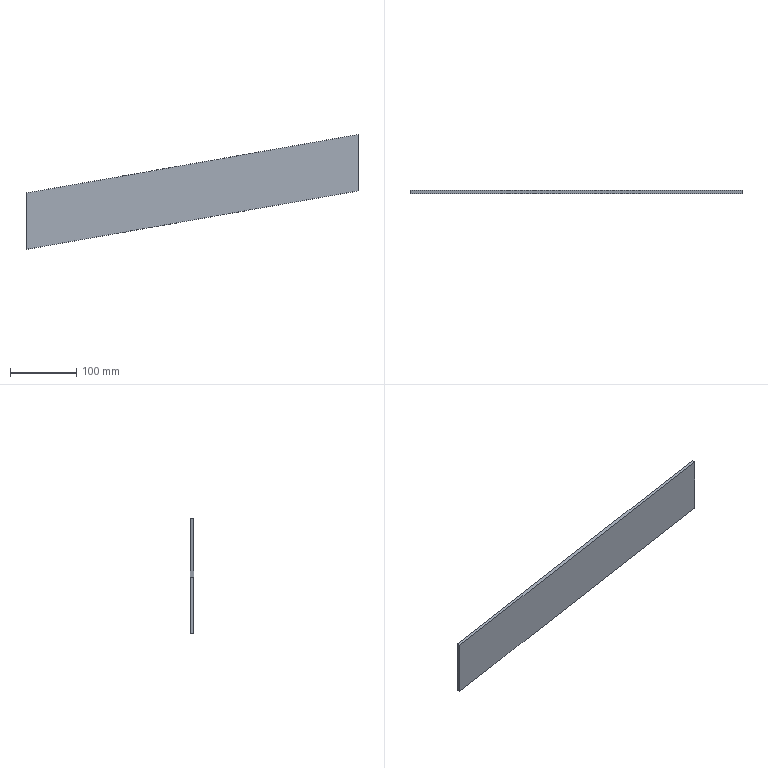Part | NX | features DATUM_CSYS 1, EXTRUDE 1, LINKED_CURVE 1 | 1 solid | 6 faces | box 500 x 5 x 173.163 mm | volume 212500 mm3 | plane 6
STEP:
#1=CARTESIAN_POINT('',(-455.,2.5,-88.163));
#2=VERTEX_POINT('',#1);
#3=CARTESIAN_POINT('',(-455.,-2.5,-88.163));
#4=VERTEX_POINT('',#3);
#5=CARTESIAN_POINT('',(-455.,0.,-88.163));
#6=DIRECTION('',(0.,-1.,0.));
#7=VECTOR('',#6,1000.);
#8=LINE('',#5,#7);
#9=EDGE_CURVE('',#2,#4,#8,.T.);
#10=ORIENTED_EDGE('',*,*,#9,.F.);
#11=CARTESIAN_POINT('',(45.,2.5,0.));
#12=VERTEX_POINT('',#11);
#13=CARTESIAN_POINT('',(-455.,2.5,-88.163));
#14=DIRECTION('',(0.9848,0.,0.1736));
#15=VECTOR('',#14,1000.);
#16=LINE('',#13,#15);
#17=EDGE_CURVE('',#2,#12,#16,.T.);
#18=ORIENTED_EDGE('',*,*,#17,.T.);
#19=CARTESIAN_POINT('',(45.,-2.5,0.));
#20=VERTEX_POINT('',#19);
#21=CARTESIAN_POINT('',(45.,0.,0.));
#22=DIRECTION('',(0.,-1.,0.));
#23=VECTOR('',#22,1000.);
#24=LINE('',#21,#23);
#25=EDGE_CURVE('',#12,#20,#24,.T.);
#26=ORIENTED_EDGE('',*,*,#25,.T.);
#27=CARTESIAN_POINT('',(-455.,-2.5,-88.163));
#28=DIRECTION('',(0.9848,0.,0.1736));
#29=VECTOR('',#28,1000.);
#30=LINE('',#27,#29);
#31=EDGE_CURVE('',#4,#20,#30,.T.);
#32=ORIENTED_EDGE('',*,*,#31,.F.);
#33=EDGE_LOOP('',(#10,#18,#26,#32));
#34=FACE_BOUND('',#33,.T.);
#35=CARTESIAN_POINT('',(-455.,0.,-88.163));
#36=DIRECTION('',(0.1736,0.,-0.9848));
#37=DIRECTION('',(0.9848,0.,0.1736));
#38=AXIS2_PLACEMENT_3D('',#35,#36,#37);
#39=PLANE('',#38);
#40=ADVANCED_FACE('',(#34),#39,.T.);
#41=ORIENTED_EDGE('',*,*,#25,.F.);
#42=CARTESIAN_POINT('',(45.,2.5,85.));
#43=VERTEX_POINT('',#42);
#44=CARTESIAN_POINT('',(45.,2.5,-88.163));
#45=DIRECTION('',(0.,0.,-1.));
#46=VECTOR('',#45,1000.);
#47=LINE('',#44,#46);
#48=EDGE_CURVE('',#12,#43,#47,.F.);
#49=ORIENTED_EDGE('',*,*,#48,.T.);
#50=CARTESIAN_POINT('',(45.,-2.5,85.));
#51=VERTEX_POINT('',#50);
#52=CARTESIAN_POINT('',(45.,0.,85.));
#53=DIRECTION('',(0.,-1.,0.));
#54=VECTOR('',#53,1000.);
#55=LINE('',#52,#54);
#56=EDGE_CURVE('',#43,#51,#55,.T.);
#57=ORIENTED_EDGE('',*,*,#56,.T.);
#58=CARTESIAN_POINT('',(45.,-2.5,-88.163));
#59=DIRECTION('',(0.,0.,-1.));
#60=VECTOR('',#59,1000.);
#61=LINE('',#58,#60);
#62=EDGE_CURVE('',#20,#51,#61,.F.);
#63=ORIENTED_EDGE('',*,*,#62,.F.);
#64=EDGE_LOOP('',(#41,#49,#57,#63));
#65=FACE_BOUND('',#64,.T.);
#66=CARTESIAN_POINT('',(45.,0.,0.));
#67=DIRECTION('',(1.,0.,0.));
#68=DIRECTION('',(0.,0.,1.));
#69=AXIS2_PLACEMENT_3D('',#66,#67,#68);
#70=PLANE('',#69);
#71=ADVANCED_FACE('',(#65),#70,.T.);
#72=ORIENTED_EDGE('',*,*,#56,.F.);
#73=CARTESIAN_POINT('',(-455.,2.5,-3.163));
#74=VERTEX_POINT('',#73);
#75=CARTESIAN_POINT('',(-455.,2.5,-3.163));
#76=DIRECTION('',(0.9848,0.,0.1736));
#77=VECTOR('',#76,1000.);
#78=LINE('',#75,#77);
#79=EDGE_CURVE('',#74,#43,#78,.T.);
#80=ORIENTED_EDGE('',*,*,#79,.F.);
#81=CARTESIAN_POINT('',(-455.,-2.5,-3.163));
#82=VERTEX_POINT('',#81);
#83=CARTESIAN_POINT('',(-455.,0.,-3.163));
#84=DIRECTION('',(0.,-1.,0.));
#85=VECTOR('',#84,1000.);
#86=LINE('',#83,#85);
#87=EDGE_CURVE('',#74,#82,#86,.T.);
#88=ORIENTED_EDGE('',*,*,#87,.T.);
#89=CARTESIAN_POINT('',(-455.,-2.5,-3.163));
#90=DIRECTION('',(0.9848,0.,0.1736));
#91=VECTOR('',#90,1000.);
#92=LINE('',#89,#91);
#93=EDGE_CURVE('',#82,#51,#92,.T.);
#94=ORIENTED_EDGE('',*,*,#93,.T.);
#95=EDGE_LOOP('',(#72,#80,#88,#94));
#96=FACE_BOUND('',#95,.T.);
#97=CARTESIAN_POINT('',(-455.,0.,-3.163));
#98=DIRECTION('',(0.1736,0.,-0.9848));
#99=DIRECTION('',(0.9848,0.,0.1736));
#100=AXIS2_PLACEMENT_3D('',#97,#98,#99);
#101=PLANE('',#100);
#102=ADVANCED_FACE('',(#96),#101,.F.);
#103=CARTESIAN_POINT('',(-455.,2.5,-88.163));
#104=DIRECTION('',(0.,0.,-1.));
#105=VECTOR('',#104,1000.);
#106=LINE('',#103,#105);
#107=EDGE_CURVE('',#2,#74,#106,.F.);
#108=ORIENTED_EDGE('',*,*,#107,.F.);
#109=ORIENTED_EDGE('',*,*,#9,.T.);
#110=CARTESIAN_POINT('',(-455.,-2.5,-88.163));
#111=DIRECTION('',(0.,0.,-1.));
#112=VECTOR('',#111,1000.);
#113=LINE('',#110,#112);
#114=EDGE_CURVE('',#4,#82,#113,.F.);
#115=ORIENTED_EDGE('',*,*,#114,.T.);
#116=ORIENTED_EDGE('',*,*,#87,.F.);
#117=EDGE_LOOP('',(#108,#109,#115,#116));
#118=FACE_BOUND('',#117,.T.);
#119=CARTESIAN_POINT('',(-455.,0.,-88.163));
#120=DIRECTION('',(1.,0.,0.));
#121=DIRECTION('',(0.,0.,1.));
#122=AXIS2_PLACEMENT_3D('',#119,#120,#121);
#123=PLANE('',#122);
#124=ADVANCED_FACE('',(#118),#123,.F.);
#125=ORIENTED_EDGE('',*,*,#93,.F.);
#126=ORIENTED_EDGE('',*,*,#114,.F.);
#127=ORIENTED_EDGE('',*,*,#31,.T.);
#128=ORIENTED_EDGE('',*,*,#62,.T.);
#129=EDGE_LOOP('',(#125,#126,#127,#128));
#130=FACE_BOUND('',#129,.T.);
#131=CARTESIAN_POINT('',(-455.,-2.5,-88.163));
#132=DIRECTION('',(0.,-1.,0.));
#133=DIRECTION('',(0.,0.,-1.));
#134=AXIS2_PLACEMENT_3D('',#131,#132,#133);
#135=PLANE('',#134);
#136=ADVANCED_FACE('',(#130),#135,.T.);
#137=ORIENTED_EDGE('',*,*,#79,.T.);
#138=ORIENTED_EDGE('',*,*,#48,.F.);
#139=ORIENTED_EDGE('',*,*,#17,.F.);
#140=ORIENTED_EDGE('',*,*,#107,.T.);
#141=EDGE_LOOP('',(#137,#138,#139,#140));
#142=FACE_BOUND('',#141,.T.);
#143=CARTESIAN_POINT('',(-455.,2.5,-88.163));
#144=DIRECTION('',(0.,-1.,0.));
#145=DIRECTION('',(0.,0.,-1.));
#146=AXIS2_PLACEMENT_3D('',#143,#144,#145);
#147=PLANE('',#146);
#148=ADVANCED_FACE('',(#142),#147,.F.);
#149=CLOSED_SHELL('',(#40,#71,#102,#124,#136,#148));
#150=MANIFOLD_SOLID_BREP('',#149);
#151=(LENGTH_UNIT()NAMED_UNIT(*)SI_UNIT(.MILLI.,.METRE.));
#152=UNCERTAINTY_MEASURE_WITH_UNIT(LENGTH_MEASURE(0.00001),#151,'','');
#153=(NAMED_UNIT(*)PLANE_ANGLE_UNIT()SI_UNIT($,.RADIAN.));
#154=(NAMED_UNIT(*)SI_UNIT($,.STERADIAN.)SOLID_ANGLE_UNIT());
#155=(GEOMETRIC_REPRESENTATION_CONTEXT(3)GLOBAL_UNCERTAINTY_ASSIGNED_CONTEXT((#152))GLOBAL_UNIT_ASSIGNED_CONTEXT((#151,#153,#154))REPRESENTATION_CONTEXT('',''));
#156=ADVANCED_BREP_SHAPE_REPRESENTATION('',(#150),#155);